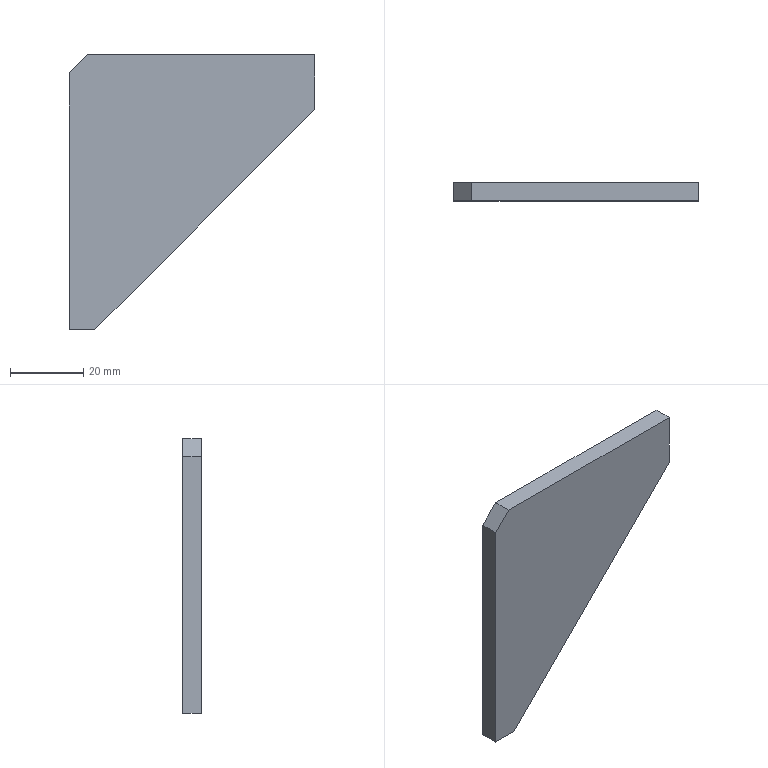Part | SolidWorks | features BaseBody 1, Chamfer 1 | 1 solid | 8 faces | box 67 x 5 x 75 mm | volume 16062 mm3 | plane 8
STEP:
#1=CARTESIAN_POINT('',(-26.5,2.5,0.));
#2=VERTEX_POINT('',#1);
#3=CARTESIAN_POINT('',(-26.5,-2.5,0.));
#4=VERTEX_POINT('',#3);
#5=CARTESIAN_POINT('',(-26.5,0.,0.));
#6=DIRECTION('',(0.,-1.,0.));
#7=VECTOR('',#6,1000.);
#8=LINE('',#5,#7);
#9=EDGE_CURVE('',#2,#4,#8,.T.);
#10=ORIENTED_EDGE('',*,*,#9,.F.);
#11=CARTESIAN_POINT('',(33.5,2.5,60.));
#12=VERTEX_POINT('',#11);
#13=CARTESIAN_POINT('',(33.5,2.5,60.));
#14=DIRECTION('',(0.7071,0.,0.7071));
#15=VECTOR('',#14,1000.);
#16=LINE('',#13,#15);
#17=EDGE_CURVE('',#2,#12,#16,.T.);
#18=ORIENTED_EDGE('',*,*,#17,.T.);
#19=CARTESIAN_POINT('',(33.5,-2.5,60.));
#20=VERTEX_POINT('',#19);
#21=CARTESIAN_POINT('',(33.5,-7.5,60.));
#22=DIRECTION('',(0.,1.,0.));
#23=VECTOR('',#22,1000.);
#24=LINE('',#21,#23);
#25=EDGE_CURVE('',#20,#12,#24,.T.);
#26=ORIENTED_EDGE('',*,*,#25,.F.);
#27=CARTESIAN_POINT('',(7.5,-2.5,34.));
#28=DIRECTION('',(0.7071,0.,0.7071));
#29=VECTOR('',#28,1000.);
#30=LINE('',#27,#29);
#31=EDGE_CURVE('',#4,#20,#30,.T.);
#32=ORIENTED_EDGE('',*,*,#31,.F.);
#33=EDGE_LOOP('',(#10,#18,#26,#32));
#34=FACE_OUTER_BOUND('',#33,.T.);
#35=CARTESIAN_POINT('',(33.5,-7.5,60.));
#36=DIRECTION('',(-0.7071,0.,0.7071));
#37=DIRECTION('',(0.,1.,0.));
#38=AXIS2_PLACEMENT_3D('',#35,#36,#37);
#39=PLANE('',#38);
#40=ADVANCED_FACE('',(#34),#39,.F.);
#41=CARTESIAN_POINT('',(-33.5,2.5,0.));
#42=VERTEX_POINT('',#41);
#43=CARTESIAN_POINT('',(-33.5,2.5,0.));
#44=DIRECTION('',(-1.,0.,0.));
#45=VECTOR('',#44,1000.);
#46=LINE('',#43,#45);
#47=EDGE_CURVE('',#2,#42,#46,.T.);
#48=ORIENTED_EDGE('',*,*,#47,.F.);
#49=ORIENTED_EDGE('',*,*,#9,.T.);
#50=CARTESIAN_POINT('',(-33.5,-2.5,0.));
#51=VERTEX_POINT('',#50);
#52=CARTESIAN_POINT('',(-33.5,-2.5,0.));
#53=DIRECTION('',(1.,0.,0.));
#54=VECTOR('',#53,1000.);
#55=LINE('',#52,#54);
#56=EDGE_CURVE('',#51,#4,#55,.T.);
#57=ORIENTED_EDGE('',*,*,#56,.F.);
#58=CARTESIAN_POINT('',(-33.5,2.5,0.));
#59=DIRECTION('',(0.,-1.,0.));
#60=VECTOR('',#59,1000.);
#61=LINE('',#58,#60);
#62=EDGE_CURVE('',#42,#51,#61,.T.);
#63=ORIENTED_EDGE('',*,*,#62,.F.);
#64=EDGE_LOOP('',(#48,#49,#57,#63));
#65=FACE_OUTER_BOUND('',#64,.T.);
#66=CARTESIAN_POINT('',(0.,0.,0.));
#67=DIRECTION('',(0.,0.,1.));
#68=DIRECTION('',(1.,0.,0.));
#69=AXIS2_PLACEMENT_3D('',#66,#67,#68);
#70=PLANE('',#69);
#71=ADVANCED_FACE('',(#65),#70,.F.);
#72=CARTESIAN_POINT('',(33.5,2.5,75.));
#73=VERTEX_POINT('',#72);
#74=CARTESIAN_POINT('',(-28.5,2.5,75.));
#75=VERTEX_POINT('',#74);
#76=CARTESIAN_POINT('',(-33.5,2.5,75.));
#77=DIRECTION('',(-1.,0.,0.));
#78=VECTOR('',#77,1000.);
#79=LINE('',#76,#78);
#80=EDGE_CURVE('',#73,#75,#79,.T.);
#81=ORIENTED_EDGE('',*,*,#80,.T.);
#82=CARTESIAN_POINT('',(-28.5,-2.5,75.));
#83=VERTEX_POINT('',#82);
#84=CARTESIAN_POINT('',(-28.5,-2.5,75.));
#85=DIRECTION('',(0.,-1.,0.));
#86=VECTOR('',#85,1000.);
#87=LINE('',#84,#86);
#88=EDGE_CURVE('',#75,#83,#87,.T.);
#89=ORIENTED_EDGE('',*,*,#88,.T.);
#90=CARTESIAN_POINT('',(33.5,-2.5,75.));
#91=VERTEX_POINT('',#90);
#92=CARTESIAN_POINT('',(-33.5,-2.5,75.));
#93=DIRECTION('',(1.,0.,0.));
#94=VECTOR('',#93,1000.);
#95=LINE('',#92,#94);
#96=EDGE_CURVE('',#83,#91,#95,.T.);
#97=ORIENTED_EDGE('',*,*,#96,.T.);
#98=CARTESIAN_POINT('',(33.5,2.5,75.));
#99=DIRECTION('',(0.,1.,0.));
#100=VECTOR('',#99,1000.);
#101=LINE('',#98,#100);
#102=EDGE_CURVE('',#91,#73,#101,.T.);
#103=ORIENTED_EDGE('',*,*,#102,.T.);
#104=EDGE_LOOP('',(#81,#89,#97,#103));
#105=FACE_OUTER_BOUND('',#104,.T.);
#106=CARTESIAN_POINT('',(0.,0.,75.));
#107=DIRECTION('',(0.,0.,1.));
#108=DIRECTION('',(1.,0.,0.));
#109=AXIS2_PLACEMENT_3D('',#106,#107,#108);
#110=PLANE('',#109);
#111=ADVANCED_FACE('',(#105),#110,.T.);
#112=ORIENTED_EDGE('',*,*,#96,.F.);
#113=CARTESIAN_POINT('',(-33.5,-2.5,70.));
#114=VERTEX_POINT('',#113);
#115=CARTESIAN_POINT('',(-28.5,-2.5,75.));
#116=DIRECTION('',(-0.7071,0.,-0.7071));
#117=VECTOR('',#116,1000.);
#118=LINE('',#115,#117);
#119=EDGE_CURVE('',#83,#114,#118,.T.);
#120=ORIENTED_EDGE('',*,*,#119,.T.);
#121=CARTESIAN_POINT('',(-33.5,-2.5,75.));
#122=DIRECTION('',(0.,0.,-1.));
#123=VECTOR('',#122,1000.);
#124=LINE('',#121,#123);
#125=EDGE_CURVE('',#114,#51,#124,.T.);
#126=ORIENTED_EDGE('',*,*,#125,.T.);
#127=ORIENTED_EDGE('',*,*,#56,.T.);
#128=ORIENTED_EDGE('',*,*,#31,.T.);
#129=CARTESIAN_POINT('',(33.5,-2.5,75.));
#130=DIRECTION('',(0.,0.,-1.));
#131=VECTOR('',#130,1000.);
#132=LINE('',#129,#131);
#133=EDGE_CURVE('',#91,#20,#132,.T.);
#134=ORIENTED_EDGE('',*,*,#133,.F.);
#135=EDGE_LOOP('',(#112,#120,#126,#127,#128,#134));
#136=FACE_OUTER_BOUND('',#135,.T.);
#137=CARTESIAN_POINT('',(-33.5,-2.5,75.));
#138=DIRECTION('',(0.,1.,0.));
#139=DIRECTION('',(0.,0.,-1.));
#140=AXIS2_PLACEMENT_3D('',#137,#138,#139);
#141=PLANE('',#140);
#142=ADVANCED_FACE('',(#136),#141,.F.);
#143=ORIENTED_EDGE('',*,*,#125,.F.);
#144=CARTESIAN_POINT('',(-33.5,2.5,70.));
#145=VERTEX_POINT('',#144);
#146=CARTESIAN_POINT('',(-33.5,2.5,70.));
#147=DIRECTION('',(0.,1.,0.));
#148=VECTOR('',#147,1000.);
#149=LINE('',#146,#148);
#150=EDGE_CURVE('',#114,#145,#149,.T.);
#151=ORIENTED_EDGE('',*,*,#150,.T.);
#152=CARTESIAN_POINT('',(-33.5,2.5,75.));
#153=DIRECTION('',(0.,0.,-1.));
#154=VECTOR('',#153,1000.);
#155=LINE('',#152,#154);
#156=EDGE_CURVE('',#145,#42,#155,.T.);
#157=ORIENTED_EDGE('',*,*,#156,.T.);
#158=ORIENTED_EDGE('',*,*,#62,.T.);
#159=EDGE_LOOP('',(#143,#151,#157,#158));
#160=FACE_OUTER_BOUND('',#159,.T.);
#161=CARTESIAN_POINT('',(-33.5,2.5,75.));
#162=DIRECTION('',(1.,0.,0.));
#163=DIRECTION('',(0.,1.,0.));
#164=AXIS2_PLACEMENT_3D('',#161,#162,#163);
#165=PLANE('',#164);
#166=ADVANCED_FACE('',(#160),#165,.F.);
#167=ORIENTED_EDGE('',*,*,#156,.F.);
#168=CARTESIAN_POINT('',(-28.5,2.5,75.));
#169=DIRECTION('',(0.7071,0.,0.7071));
#170=VECTOR('',#169,1000.);
#171=LINE('',#168,#170);
#172=EDGE_CURVE('',#145,#75,#171,.T.);
#173=ORIENTED_EDGE('',*,*,#172,.T.);
#174=ORIENTED_EDGE('',*,*,#80,.F.);
#175=CARTESIAN_POINT('',(33.5,2.5,75.));
#176=DIRECTION('',(0.,0.,-1.));
#177=VECTOR('',#176,1000.);
#178=LINE('',#175,#177);
#179=EDGE_CURVE('',#73,#12,#178,.T.);
#180=ORIENTED_EDGE('',*,*,#179,.T.);
#181=ORIENTED_EDGE('',*,*,#17,.F.);
#182=ORIENTED_EDGE('',*,*,#47,.T.);
#183=EDGE_LOOP('',(#167,#173,#174,#180,#181,#182));
#184=FACE_OUTER_BOUND('',#183,.T.);
#185=CARTESIAN_POINT('',(-33.5,2.5,75.));
#186=DIRECTION('',(0.,-1.,0.));
#187=DIRECTION('',(0.,0.,-1.));
#188=AXIS2_PLACEMENT_3D('',#185,#186,#187);
#189=PLANE('',#188);
#190=ADVANCED_FACE('',(#184),#189,.F.);
#191=ORIENTED_EDGE('',*,*,#133,.T.);
#192=ORIENTED_EDGE('',*,*,#25,.T.);
#193=ORIENTED_EDGE('',*,*,#179,.F.);
#194=ORIENTED_EDGE('',*,*,#102,.F.);
#195=EDGE_LOOP('',(#191,#192,#193,#194));
#196=FACE_OUTER_BOUND('',#195,.T.);
#197=CARTESIAN_POINT('',(33.5,2.5,75.));
#198=DIRECTION('',(-1.,0.,0.));
#199=DIRECTION('',(0.,1.,0.));
#200=AXIS2_PLACEMENT_3D('',#197,#198,#199);
#201=PLANE('',#200);
#202=ADVANCED_FACE('',(#196),#201,.F.);
#203=ORIENTED_EDGE('',*,*,#172,.F.);
#204=ORIENTED_EDGE('',*,*,#150,.F.);
#205=ORIENTED_EDGE('',*,*,#119,.F.);
#206=ORIENTED_EDGE('',*,*,#88,.F.);
#207=EDGE_LOOP('',(#203,#204,#205,#206));
#208=FACE_OUTER_BOUND('',#207,.T.);
#209=CARTESIAN_POINT('',(-28.5,0.,75.));
#210=DIRECTION('',(-0.7071,0.,0.7071));
#211=DIRECTION('',(0.,1.,0.));
#212=AXIS2_PLACEMENT_3D('',#209,#210,#211);
#213=PLANE('',#212);
#214=ADVANCED_FACE('',(#208),#213,.T.);
#215=CLOSED_SHELL('',(#40,#71,#111,#142,#166,#190,#202,#214));
#216=MANIFOLD_SOLID_BREP('',#215);
#217=CARTESIAN_POINT('',(0.,0.,0.));
#218=DIRECTION('',(0.,0.,1.));
#219=DIRECTION('',(1.,0.,0.));
#220=AXIS2_PLACEMENT_3D('',#217,#218,#219);
#221=(LENGTH_UNIT()NAMED_UNIT(*)SI_UNIT(.MILLI.,.METRE.));
#222=UNCERTAINTY_MEASURE_WITH_UNIT(LENGTH_MEASURE(0.00001),#221,'','');
#223=(NAMED_UNIT(*)PLANE_ANGLE_UNIT()SI_UNIT($,.RADIAN.));
#224=(NAMED_UNIT(*)SI_UNIT($,.STERADIAN.)SOLID_ANGLE_UNIT());
#225=(GEOMETRIC_REPRESENTATION_CONTEXT(3)GLOBAL_UNCERTAINTY_ASSIGNED_CONTEXT((#222))GLOBAL_UNIT_ASSIGNED_CONTEXT((#221,#223,#224))REPRESENTATION_CONTEXT('',''));
#226=ADVANCED_BREP_SHAPE_REPRESENTATION('',(#216,#220),#225);